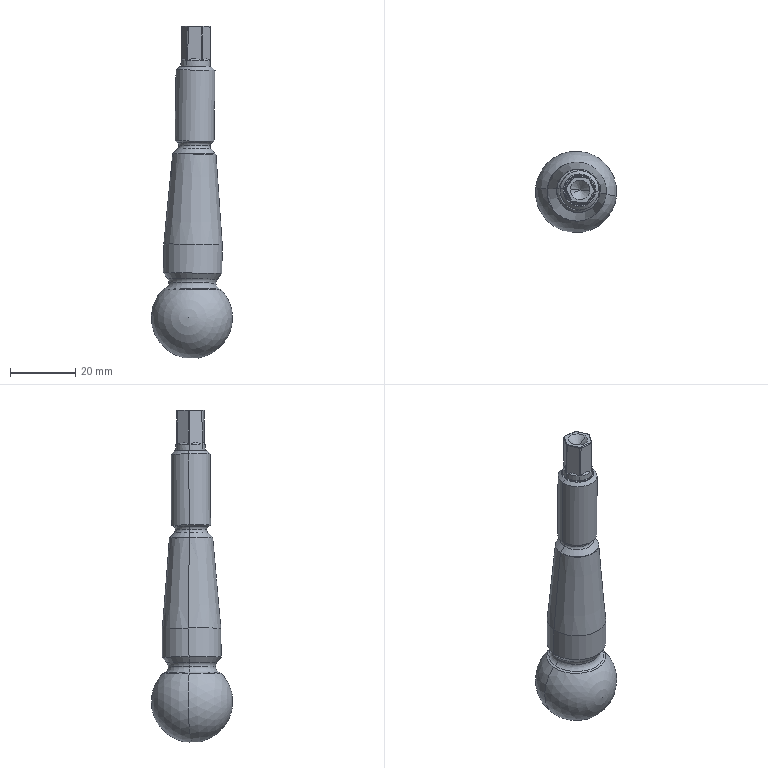Part | SolidWorks | features BaseBody 1 | 1 solid | 66 faces | box 25 x 25 x 101.883 mm | volume 19881 mm3 | torus 21 | cone 20 | cylinder 14 | plane 9 | sphere 2 | commonest cylinder face diameters 0.4 x6 9 x4 12 x2 18 x2